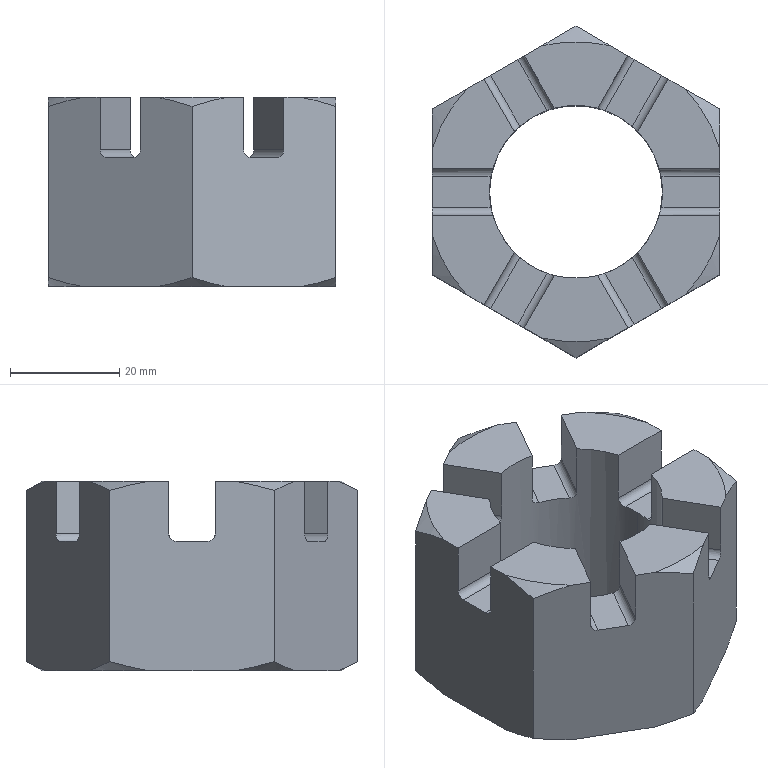Part | SolidWorks | features Cut 3, Chamfer 1, CirPattern 1, Extrusion 1 | 1 solid | 59 faces | box 52.646 x 60.79 x 34.7 mm | volume 49893 mm3 | plane 31 | cone 14 | cylinder 14 | commonest cylinder face diameters 2.75 x12 31.67 x2